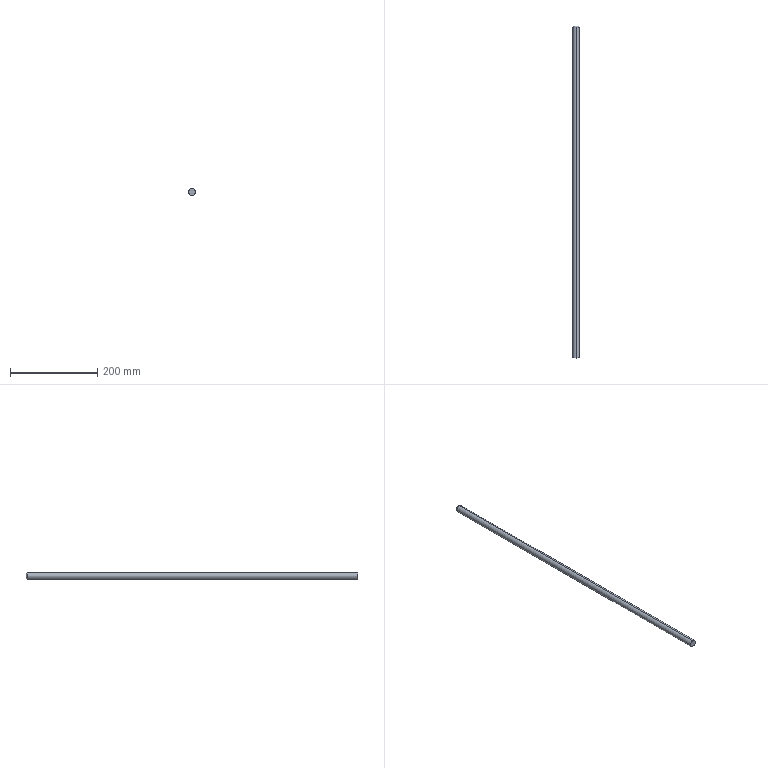Part | SolidWorks | features Chamfer 1, Extrusion 1 | 1 solid | 6 faces | box 16 x 759 x 16 mm | volume 152408 mm3 | cone 2 | cylinder 2 | plane 2 | commonest cylinder face diameters 16 x2
STEP:
#1=CARTESIAN_POINT('',(0.,759.,5.));
#2=VERTEX_POINT('',#1);
#3=CARTESIAN_POINT('',(0.,759.,-5.));
#4=VERTEX_POINT('',#3);
#5=CARTESIAN_POINT('',(0.,759.,0.));
#6=DIRECTION('',(0.,1.,0.));
#7=DIRECTION('',(0.,0.,1.));
#8=AXIS2_PLACEMENT_3D('',#5,#6,#7);
#9=CIRCLE('',#8,5.);
#10=EDGE_CURVE('',#2,#4,#9,.T.);
#11=ORIENTED_EDGE('',*,*,#10,.F.);
#12=CARTESIAN_POINT('',(0.,756.,8.));
#13=VERTEX_POINT('',#12);
#14=CARTESIAN_POINT('',(0.,759.,5.));
#15=DIRECTION('',(0.,-0.7071,0.7071));
#16=VECTOR('',#15,1000.);
#17=LINE('',#14,#16);
#18=EDGE_CURVE('',#2,#13,#17,.T.);
#19=ORIENTED_EDGE('',*,*,#18,.T.);
#20=CARTESIAN_POINT('',(0.,756.,-8.));
#21=VERTEX_POINT('',#20);
#22=CARTESIAN_POINT('',(0.,756.,0.));
#23=DIRECTION('',(0.,-1.,0.));
#24=DIRECTION('',(0.,0.,1.));
#25=AXIS2_PLACEMENT_3D('',#22,#23,#24);
#26=CIRCLE('',#25,8.);
#27=EDGE_CURVE('',#21,#13,#26,.T.);
#28=ORIENTED_EDGE('',*,*,#27,.F.);
#29=CARTESIAN_POINT('',(0.,759.,-5.));
#30=DIRECTION('',(0.,-0.7071,-0.7071));
#31=VECTOR('',#30,1000.);
#32=LINE('',#29,#31);
#33=EDGE_CURVE('',#4,#21,#32,.T.);
#34=ORIENTED_EDGE('',*,*,#33,.F.);
#35=EDGE_LOOP('',(#11,#19,#28,#34));
#36=FACE_OUTER_BOUND('',#35,.T.);
#37=CARTESIAN_POINT('',(0.,759.,0.));
#38=DIRECTION('',(0.,-1.,0.));
#39=DIRECTION('',(0.,0.,-1.));
#40=AXIS2_PLACEMENT_3D('',#37,#38,#39);
#41=CONICAL_SURFACE('',#40,5.,0.7854);
#42=ADVANCED_FACE('',(#36),#41,.T.);
#43=ORIENTED_EDGE('',*,*,#27,.T.);
#44=CARTESIAN_POINT('',(0.,0.,8.));
#45=VERTEX_POINT('',#44);
#46=CARTESIAN_POINT('',(0.,759.,8.));
#47=DIRECTION('',(0.,-1.,0.));
#48=VECTOR('',#47,1000.);
#49=LINE('',#46,#48);
#50=EDGE_CURVE('',#13,#45,#49,.T.);
#51=ORIENTED_EDGE('',*,*,#50,.T.);
#52=CARTESIAN_POINT('',(0.,0.,-8.));
#53=VERTEX_POINT('',#52);
#54=CARTESIAN_POINT('',(0.,0.,0.));
#55=DIRECTION('',(0.,1.,0.));
#56=DIRECTION('',(0.,0.,1.));
#57=AXIS2_PLACEMENT_3D('',#54,#55,#56);
#58=CIRCLE('',#57,8.);
#59=EDGE_CURVE('',#45,#53,#58,.T.);
#60=ORIENTED_EDGE('',*,*,#59,.T.);
#61=CARTESIAN_POINT('',(0.,759.,-8.));
#62=DIRECTION('',(0.,-1.,0.));
#63=VECTOR('',#62,1000.);
#64=LINE('',#61,#63);
#65=EDGE_CURVE('',#21,#53,#64,.T.);
#66=ORIENTED_EDGE('',*,*,#65,.F.);
#67=EDGE_LOOP('',(#43,#51,#60,#66));
#68=FACE_OUTER_BOUND('',#67,.T.);
#69=CARTESIAN_POINT('',(0.,759.,0.));
#70=DIRECTION('',(0.,-1.,0.));
#71=DIRECTION('',(0.,0.,-1.));
#72=AXIS2_PLACEMENT_3D('',#69,#70,#71);
#73=CYLINDRICAL_SURFACE('',#72,8.);
#74=ADVANCED_FACE('',(#68),#73,.T.);
#75=ORIENTED_EDGE('',*,*,#50,.F.);
#76=CARTESIAN_POINT('',(0.,756.,0.));
#77=DIRECTION('',(0.,-1.,0.));
#78=DIRECTION('',(0.,0.,1.));
#79=AXIS2_PLACEMENT_3D('',#76,#77,#78);
#80=CIRCLE('',#79,8.);
#81=EDGE_CURVE('',#13,#21,#80,.T.);
#82=ORIENTED_EDGE('',*,*,#81,.T.);
#83=ORIENTED_EDGE('',*,*,#65,.T.);
#84=CARTESIAN_POINT('',(0.,0.,0.));
#85=DIRECTION('',(0.,1.,0.));
#86=DIRECTION('',(0.,0.,1.));
#87=AXIS2_PLACEMENT_3D('',#84,#85,#86);
#88=CIRCLE('',#87,8.);
#89=EDGE_CURVE('',#53,#45,#88,.T.);
#90=ORIENTED_EDGE('',*,*,#89,.T.);
#91=EDGE_LOOP('',(#75,#82,#83,#90));
#92=FACE_OUTER_BOUND('',#91,.T.);
#93=CARTESIAN_POINT('',(0.,759.,0.));
#94=DIRECTION('',(0.,-1.,0.));
#95=DIRECTION('',(0.,0.,-1.));
#96=AXIS2_PLACEMENT_3D('',#93,#94,#95);
#97=CYLINDRICAL_SURFACE('',#96,8.);
#98=ADVANCED_FACE('',(#92),#97,.T.);
#99=CARTESIAN_POINT('',(0.,759.,0.));
#100=DIRECTION('',(0.,1.,0.));
#101=DIRECTION('',(0.,0.,1.));
#102=AXIS2_PLACEMENT_3D('',#99,#100,#101);
#103=CIRCLE('',#102,5.);
#104=EDGE_CURVE('',#4,#2,#103,.T.);
#105=ORIENTED_EDGE('',*,*,#104,.T.);
#106=ORIENTED_EDGE('',*,*,#10,.T.);
#107=EDGE_LOOP('',(#105,#106));
#108=FACE_OUTER_BOUND('',#107,.T.);
#109=CARTESIAN_POINT('',(0.,759.,0.));
#110=DIRECTION('',(0.,1.,0.));
#111=DIRECTION('',(0.,0.,1.));
#112=AXIS2_PLACEMENT_3D('',#109,#110,#111);
#113=PLANE('',#112);
#114=ADVANCED_FACE('',(#108),#113,.T.);
#115=ORIENTED_EDGE('',*,*,#89,.F.);
#116=ORIENTED_EDGE('',*,*,#59,.F.);
#117=EDGE_LOOP('',(#115,#116));
#118=FACE_OUTER_BOUND('',#117,.T.);
#119=CARTESIAN_POINT('',(0.,0.,0.));
#120=DIRECTION('',(0.,1.,0.));
#121=DIRECTION('',(0.,0.,1.));
#122=AXIS2_PLACEMENT_3D('',#119,#120,#121);
#123=PLANE('',#122);
#124=ADVANCED_FACE('',(#118),#123,.F.);
#125=ORIENTED_EDGE('',*,*,#18,.F.);
#126=ORIENTED_EDGE('',*,*,#104,.F.);
#127=ORIENTED_EDGE('',*,*,#33,.T.);
#128=ORIENTED_EDGE('',*,*,#81,.F.);
#129=EDGE_LOOP('',(#125,#126,#127,#128));
#130=FACE_OUTER_BOUND('',#129,.T.);
#131=CARTESIAN_POINT('',(0.,759.,0.));
#132=DIRECTION('',(0.,-1.,0.));
#133=DIRECTION('',(0.,0.,-1.));
#134=AXIS2_PLACEMENT_3D('',#131,#132,#133);
#135=CONICAL_SURFACE('',#134,5.,0.7854);
#136=ADVANCED_FACE('',(#130),#135,.T.);
#137=CLOSED_SHELL('',(#42,#74,#98,#114,#124,#136));
#138=MANIFOLD_SOLID_BREP('',#137);
#139=CARTESIAN_POINT('',(0.,0.,0.));
#140=DIRECTION('',(0.,0.,1.));
#141=DIRECTION('',(1.,0.,0.));
#142=AXIS2_PLACEMENT_3D('',#139,#140,#141);
#143=(LENGTH_UNIT()NAMED_UNIT(*)SI_UNIT(.MILLI.,.METRE.));
#144=UNCERTAINTY_MEASURE_WITH_UNIT(LENGTH_MEASURE(0.00001),#143,'','');
#145=(NAMED_UNIT(*)PLANE_ANGLE_UNIT()SI_UNIT($,.RADIAN.));
#146=(NAMED_UNIT(*)SI_UNIT($,.STERADIAN.)SOLID_ANGLE_UNIT());
#147=(GEOMETRIC_REPRESENTATION_CONTEXT(3)GLOBAL_UNCERTAINTY_ASSIGNED_CONTEXT((#144))GLOBAL_UNIT_ASSIGNED_CONTEXT((#143,#145,#146))REPRESENTATION_CONTEXT('',''));
#148=ADVANCED_BREP_SHAPE_REPRESENTATION('',(#138,#142),#147);